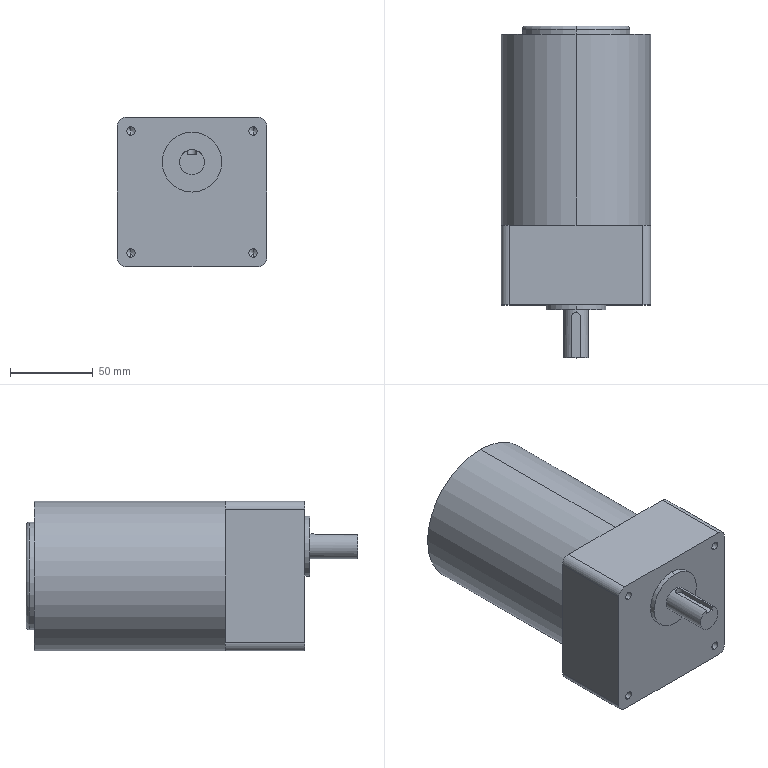Part | SolidWorks | features ICE 6, Fillet 2, CirPattern 1, Extrusion 1, HoleWzd 1, RefAxis 1 | 1 solid | 47 faces | box 90 x 200 x 90 mm | volume 1142205 mm3 | cylinder 21 | plane 16 | cone 8 | torus 2 | commonest cylinder face diameters 5 x9 10 x4 15 x2 36 x2 65 x2 90 x2
STEP:
#1=CARTESIAN_POINT('',(0.,166.,-32.5));
#2=VERTEX_POINT('',#1);
#3=CARTESIAN_POINT('',(0.,166.,32.5));
#4=VERTEX_POINT('',#3);
#5=CARTESIAN_POINT('',(0.,166.,0.));
#6=DIRECTION('',(0.,-1.,0.));
#7=DIRECTION('',(0.,0.,1.));
#8=AXIS2_PLACEMENT_3D('',#5,#6,#7);
#9=CIRCLE('',#8,32.5);
#10=EDGE_CURVE('',#2,#4,#9,.T.);
#11=ORIENTED_EDGE('',*,*,#10,.F.);
#12=CARTESIAN_POINT('',(0.,168.,-30.5));
#13=VERTEX_POINT('',#12);
#14=CARTESIAN_POINT('',(0.,166.,-30.5));
#15=DIRECTION('',(1.,0.,0.));
#16=DIRECTION('',(0.,0.,-1.));
#17=AXIS2_PLACEMENT_3D('',#14,#15,#16);
#18=CIRCLE('',#17,2.);
#19=EDGE_CURVE('',#2,#13,#18,.T.);
#20=ORIENTED_EDGE('',*,*,#19,.T.);
#21=CARTESIAN_POINT('',(0.,168.,30.5));
#22=VERTEX_POINT('',#21);
#23=CARTESIAN_POINT('',(0.,168.,0.));
#24=DIRECTION('',(0.,1.,0.));
#25=DIRECTION('',(0.,0.,1.));
#26=AXIS2_PLACEMENT_3D('',#23,#24,#25);
#27=CIRCLE('',#26,30.5);
#28=EDGE_CURVE('',#22,#13,#27,.T.);
#29=ORIENTED_EDGE('',*,*,#28,.F.);
#30=CARTESIAN_POINT('',(0.,166.,30.5));
#31=DIRECTION('',(-1.,0.,0.));
#32=DIRECTION('',(0.,0.,1.));
#33=AXIS2_PLACEMENT_3D('',#30,#31,#32);
#34=CIRCLE('',#33,2.);
#35=EDGE_CURVE('',#4,#22,#34,.T.);
#36=ORIENTED_EDGE('',*,*,#35,.F.);
#37=EDGE_LOOP('',(#11,#20,#29,#36));
#38=FACE_OUTER_BOUND('',#37,.T.);
#39=CARTESIAN_POINT('',(0.,166.,0.));
#40=DIRECTION('',(0.,1.,0.));
#41=DIRECTION('',(0.,0.,1.));
#42=AXIS2_PLACEMENT_3D('',#39,#40,#41);
#43=TOROIDAL_SURFACE('',#42,30.5,2.);
#44=ADVANCED_FACE('',(#38),#43,.T.);
#45=CARTESIAN_POINT('',(0.,163.,45.));
#46=VERTEX_POINT('',#45);
#47=CARTESIAN_POINT('',(0.,163.,-45.));
#48=VERTEX_POINT('',#47);
#49=CARTESIAN_POINT('',(0.,163.,0.));
#50=DIRECTION('',(0.,1.,0.));
#51=DIRECTION('',(0.,0.,1.));
#52=AXIS2_PLACEMENT_3D('',#49,#50,#51);
#53=CIRCLE('',#52,45.);
#54=EDGE_CURVE('',#46,#48,#53,.T.);
#55=ORIENTED_EDGE('',*,*,#54,.F.);
#56=CARTESIAN_POINT('',(0.,48.,45.));
#57=VERTEX_POINT('',#56);
#58=CARTESIAN_POINT('',(0.,163.,45.));
#59=DIRECTION('',(0.,-1.,0.));
#60=VECTOR('',#59,1000.);
#61=LINE('',#58,#60);
#62=EDGE_CURVE('',#46,#57,#61,.T.);
#63=ORIENTED_EDGE('',*,*,#62,.T.);
#64=CARTESIAN_POINT('',(45.,48.,0.));
#65=VERTEX_POINT('',#64);
#66=CARTESIAN_POINT('',(0.,48.,0.));
#67=DIRECTION('',(0.,1.,0.));
#68=DIRECTION('',(0.,0.,1.));
#69=AXIS2_PLACEMENT_3D('',#66,#67,#68);
#70=CIRCLE('',#69,45.);
#71=EDGE_CURVE('',#57,#65,#70,.T.);
#72=ORIENTED_EDGE('',*,*,#71,.T.);
#73=CARTESIAN_POINT('',(0.,48.,-45.));
#74=VERTEX_POINT('',#73);
#75=CARTESIAN_POINT('',(0.,48.,0.));
#76=DIRECTION('',(0.,1.,0.));
#77=DIRECTION('',(0.,0.,1.));
#78=AXIS2_PLACEMENT_3D('',#75,#76,#77);
#79=CIRCLE('',#78,45.);
#80=EDGE_CURVE('',#65,#74,#79,.T.);
#81=ORIENTED_EDGE('',*,*,#80,.T.);
#82=CARTESIAN_POINT('',(0.,163.,-45.));
#83=DIRECTION('',(0.,-1.,0.));
#84=VECTOR('',#83,1000.);
#85=LINE('',#82,#84);
#86=EDGE_CURVE('',#48,#74,#85,.T.);
#87=ORIENTED_EDGE('',*,*,#86,.F.);
#88=EDGE_LOOP('',(#55,#63,#72,#81,#87));
#89=FACE_OUTER_BOUND('',#88,.T.);
#90=CARTESIAN_POINT('',(0.,163.,0.));
#91=DIRECTION('',(0.,-1.,0.));
#92=DIRECTION('',(0.,0.,-1.));
#93=AXIS2_PLACEMENT_3D('',#90,#91,#92);
#94=CYLINDRICAL_SURFACE('',#93,45.);
#95=ADVANCED_FACE('',(#89),#94,.T.);
#96=ORIENTED_EDGE('',*,*,#10,.T.);
#97=CARTESIAN_POINT('',(0.,163.,32.5));
#98=VERTEX_POINT('',#97);
#99=CARTESIAN_POINT('',(0.,168.,32.5));
#100=DIRECTION('',(0.,-1.,0.));
#101=VECTOR('',#100,1000.);
#102=LINE('',#99,#101);
#103=EDGE_CURVE('',#4,#98,#102,.T.);
#104=ORIENTED_EDGE('',*,*,#103,.T.);
#105=CARTESIAN_POINT('',(0.,163.,-32.5));
#106=VERTEX_POINT('',#105);
#107=CARTESIAN_POINT('',(0.,163.,0.));
#108=DIRECTION('',(0.,1.,0.));
#109=DIRECTION('',(0.,0.,1.));
#110=AXIS2_PLACEMENT_3D('',#107,#108,#109);
#111=CIRCLE('',#110,32.5);
#112=EDGE_CURVE('',#98,#106,#111,.T.);
#113=ORIENTED_EDGE('',*,*,#112,.T.);
#114=CARTESIAN_POINT('',(0.,168.,-32.5));
#115=DIRECTION('',(0.,-1.,0.));
#116=VECTOR('',#115,1000.);
#117=LINE('',#114,#116);
#118=EDGE_CURVE('',#2,#106,#117,.T.);
#119=ORIENTED_EDGE('',*,*,#118,.F.);
#120=EDGE_LOOP('',(#96,#104,#113,#119));
#121=FACE_OUTER_BOUND('',#120,.T.);
#122=CARTESIAN_POINT('',(0.,168.,0.));
#123=DIRECTION('',(0.,-1.,0.));
#124=DIRECTION('',(0.,0.,-1.));
#125=AXIS2_PLACEMENT_3D('',#122,#123,#124);
#126=CYLINDRICAL_SURFACE('',#125,32.5);
#127=ADVANCED_FACE('',(#121),#126,.T.);
#128=CARTESIAN_POINT('',(-36.77,17.,39.27));
#129=VERTEX_POINT('',#128);
#130=CARTESIAN_POINT('',(-36.77,17.,34.27));
#131=VERTEX_POINT('',#130);
#132=CARTESIAN_POINT('',(-36.77,17.,36.77));
#133=DIRECTION('',(0.,-1.,0.));
#134=DIRECTION('',(0.,0.,-1.));
#135=AXIS2_PLACEMENT_3D('',#132,#133,#134);
#136=CIRCLE('',#135,2.5);
#137=EDGE_CURVE('',#129,#131,#136,.T.);
#138=ORIENTED_EDGE('',*,*,#137,.F.);
#139=CARTESIAN_POINT('',(-36.77,0.,39.27));
#140=VERTEX_POINT('',#139);
#141=CARTESIAN_POINT('',(-36.77,0.,39.27));
#142=DIRECTION('',(0.,-1.,0.));
#143=VECTOR('',#142,1000.);
#144=LINE('',#141,#143);
#145=EDGE_CURVE('',#129,#140,#144,.T.);
#146=ORIENTED_EDGE('',*,*,#145,.T.);
#147=CARTESIAN_POINT('',(-36.77,0.,34.27));
#148=VERTEX_POINT('',#147);
#149=CARTESIAN_POINT('',(-36.77,0.,36.77));
#150=DIRECTION('',(0.,-1.,0.));
#151=DIRECTION('',(0.,0.,-1.));
#152=AXIS2_PLACEMENT_3D('',#149,#150,#151);
#153=CIRCLE('',#152,2.5);
#154=EDGE_CURVE('',#140,#148,#153,.T.);
#155=ORIENTED_EDGE('',*,*,#154,.T.);
#156=CARTESIAN_POINT('',(-36.77,0.,34.27));
#157=DIRECTION('',(0.,-1.,0.));
#158=VECTOR('',#157,1000.);
#159=LINE('',#156,#158);
#160=EDGE_CURVE('',#131,#148,#159,.T.);
#161=ORIENTED_EDGE('',*,*,#160,.F.);
#162=EDGE_LOOP('',(#138,#146,#155,#161));
#163=FACE_OUTER_BOUND('',#162,.T.);
#164=CARTESIAN_POINT('',(-36.77,0.,36.77));
#165=DIRECTION('',(0.,-1.,0.));
#166=DIRECTION('',(0.,0.,-1.));
#167=AXIS2_PLACEMENT_3D('',#164,#165,#166);
#168=CYLINDRICAL_SURFACE('',#167,2.5);
#169=ADVANCED_FACE('',(#163),#168,.F.);
#170=CARTESIAN_POINT('',(-36.77,18.502,36.77));
#171=VERTEX_POINT('',#170);
#172=CARTESIAN_POINT('',(-36.77,17.,34.27));
#173=DIRECTION('',(0.,-0.515,-0.8572));
#174=VECTOR('',#173,1000.);
#175=LINE('',#172,#174);
#176=EDGE_CURVE('',#171,#131,#175,.T.);
#177=ORIENTED_EDGE('',*,*,#176,.F.);
#178=CARTESIAN_POINT('',(-36.77,17.,39.27));
#179=DIRECTION('',(0.,-0.515,0.8572));
#180=VECTOR('',#179,1000.);
#181=LINE('',#178,#180);
#182=EDGE_CURVE('',#171,#129,#181,.T.);
#183=ORIENTED_EDGE('',*,*,#182,.T.);
#184=ORIENTED_EDGE('',*,*,#137,.T.);
#185=EDGE_LOOP('',(#177,#183,#184));
#186=FACE_OUTER_BOUND('',#185,.T.);
#187=CARTESIAN_POINT('',(-36.77,17.,36.77));
#188=DIRECTION('',(0.,-1.,0.));
#189=DIRECTION('',(0.,0.,-1.));
#190=AXIS2_PLACEMENT_3D('',#187,#188,#189);
#191=CONICAL_SURFACE('',#190,2.5,1.03);
#192=ADVANCED_FACE('',(#186),#191,.F.);
#193=CARTESIAN_POINT('',(-36.77,17.,-34.27));
#194=VERTEX_POINT('',#193);
#195=CARTESIAN_POINT('',(-36.77,17.,-39.27));
#196=VERTEX_POINT('',#195);
#197=CARTESIAN_POINT('',(-36.77,17.,-36.77));
#198=DIRECTION('',(0.,-1.,0.));
#199=DIRECTION('',(0.,0.,-1.));
#200=AXIS2_PLACEMENT_3D('',#197,#198,#199);
#201=CIRCLE('',#200,2.5);
#202=EDGE_CURVE('',#194,#196,#201,.T.);
#203=ORIENTED_EDGE('',*,*,#202,.F.);
#204=CARTESIAN_POINT('',(-36.77,0.,-34.27));
#205=VERTEX_POINT('',#204);
#206=CARTESIAN_POINT('',(-36.77,0.,-34.27));
#207=DIRECTION('',(0.,-1.,0.));
#208=VECTOR('',#207,1000.);
#209=LINE('',#206,#208);
#210=EDGE_CURVE('',#194,#205,#209,.T.);
#211=ORIENTED_EDGE('',*,*,#210,.T.);
#212=CARTESIAN_POINT('',(-36.77,0.,-39.27));
#213=VERTEX_POINT('',#212);
#214=CARTESIAN_POINT('',(-36.77,0.,-36.77));
#215=DIRECTION('',(0.,-1.,0.));
#216=DIRECTION('',(0.,0.,-1.));
#217=AXIS2_PLACEMENT_3D('',#214,#215,#216);
#218=CIRCLE('',#217,2.5);
#219=EDGE_CURVE('',#205,#213,#218,.T.);
#220=ORIENTED_EDGE('',*,*,#219,.T.);
#221=CARTESIAN_POINT('',(-36.77,0.,-39.27));
#222=DIRECTION('',(0.,-1.,0.));
#223=VECTOR('',#222,1000.);
#224=LINE('',#221,#223);
#225=EDGE_CURVE('',#196,#213,#224,.T.);
#226=ORIENTED_EDGE('',*,*,#225,.F.);
#227=EDGE_LOOP('',(#203,#211,#220,#226));
#228=FACE_OUTER_BOUND('',#227,.T.);
#229=CARTESIAN_POINT('',(-36.77,0.,-36.77));
#230=DIRECTION('',(0.,-1.,0.));
#231=DIRECTION('',(0.,0.,-1.));
#232=AXIS2_PLACEMENT_3D('',#229,#230,#231);
#233=CYLINDRICAL_SURFACE('',#232,2.5);
#234=ADVANCED_FACE('',(#228),#233,.F.);
#235=CARTESIAN_POINT('',(-36.77,18.502,-36.77));
#236=VERTEX_POINT('',#235);
#237=CARTESIAN_POINT('',(-36.77,17.,-39.27));
#238=DIRECTION('',(0.,-0.515,-0.8572));
#239=VECTOR('',#238,1000.);
#240=LINE('',#237,#239);
#241=EDGE_CURVE('',#236,#196,#240,.T.);
#242=ORIENTED_EDGE('',*,*,#241,.F.);
#243=CARTESIAN_POINT('',(-36.77,17.,-34.27));
#244=DIRECTION('',(0.,-0.515,0.8572));
#245=VECTOR('',#244,1000.);
#246=LINE('',#243,#245);
#247=EDGE_CURVE('',#236,#194,#246,.T.);
#248=ORIENTED_EDGE('',*,*,#247,.T.);
#249=ORIENTED_EDGE('',*,*,#202,.T.);
#250=EDGE_LOOP('',(#242,#248,#249));
#251=FACE_OUTER_BOUND('',#250,.T.);
#252=CARTESIAN_POINT('',(-36.77,17.,-36.77));
#253=DIRECTION('',(0.,-1.,0.));
#254=DIRECTION('',(0.,0.,-1.));
#255=AXIS2_PLACEMENT_3D('',#252,#253,#254);
#256=CONICAL_SURFACE('',#255,2.5,1.03);
#257=ADVANCED_FACE('',(#251),#256,.F.);
#258=CARTESIAN_POINT('',(36.77,17.,-34.27));
#259=VERTEX_POINT('',#258);
#260=CARTESIAN_POINT('',(36.77,17.,-39.27));
#261=VERTEX_POINT('',#260);
#262=CARTESIAN_POINT('',(36.77,17.,-36.77));
#263=DIRECTION('',(0.,-1.,0.));
#264=DIRECTION('',(0.,0.,-1.));
#265=AXIS2_PLACEMENT_3D('',#262,#263,#264);
#266=CIRCLE('',#265,2.5);
#267=EDGE_CURVE('',#259,#261,#266,.T.);
#268=ORIENTED_EDGE('',*,*,#267,.F.);
#269=CARTESIAN_POINT('',(36.77,0.,-34.27));
#270=VERTEX_POINT('',#269);
#271=CARTESIAN_POINT('',(36.77,0.,-34.27));
#272=DIRECTION('',(0.,-1.,0.));
#273=VECTOR('',#272,1000.);
#274=LINE('',#271,#273);
#275=EDGE_CURVE('',#259,#270,#274,.T.);
#276=ORIENTED_EDGE('',*,*,#275,.T.);
#277=CARTESIAN_POINT('',(36.77,0.,-39.27));
#278=VERTEX_POINT('',#277);
#279=CARTESIAN_POINT('',(36.77,0.,-36.77));
#280=DIRECTION('',(0.,-1.,0.));
#281=DIRECTION('',(0.,0.,-1.));
#282=AXIS2_PLACEMENT_3D('',#279,#280,#281);
#283=CIRCLE('',#282,2.5);
#284=EDGE_CURVE('',#270,#278,#283,.T.);
#285=ORIENTED_EDGE('',*,*,#284,.T.);
#286=CARTESIAN_POINT('',(36.77,0.,-39.27));
#287=DIRECTION('',(0.,-1.,0.));
#288=VECTOR('',#287,1000.);
#289=LINE('',#286,#288);
#290=EDGE_CURVE('',#261,#278,#289,.T.);
#291=ORIENTED_EDGE('',*,*,#290,.F.);
#292=EDGE_LOOP('',(#268,#276,#285,#291));
#293=FACE_OUTER_BOUND('',#292,.T.);
#294=CARTESIAN_POINT('',(36.77,0.,-36.77));
#295=DIRECTION('',(0.,-1.,0.));
#296=DIRECTION('',(0.,0.,-1.));
#297=AXIS2_PLACEMENT_3D('',#294,#295,#296);
#298=CYLINDRICAL_SURFACE('',#297,2.5);
#299=ADVANCED_FACE('',(#293),#298,.F.);
#300=CARTESIAN_POINT('',(36.77,18.502,-36.77));
#301=VERTEX_POINT('',#300);
#302=CARTESIAN_POINT('',(36.77,17.,-39.27));
#303=DIRECTION('',(0.,-0.515,-0.8572));
#304=VECTOR('',#303,1000.);
#305=LINE('',#302,#304);
#306=EDGE_CURVE('',#301,#261,#305,.T.);
#307=ORIENTED_EDGE('',*,*,#306,.F.);
#308=CARTESIAN_POINT('',(36.77,17.,-34.27));
#309=DIRECTION('',(0.,-0.515,0.8572));
#310=VECTOR('',#309,1000.);
#311=LINE('',#308,#310);
#312=EDGE_CURVE('',#301,#259,#311,.T.);
#313=ORIENTED_EDGE('',*,*,#312,.T.);
#314=ORIENTED_EDGE('',*,*,#267,.T.);
#315=EDGE_LOOP('',(#307,#313,#314));
#316=FACE_OUTER_BOUND('',#315,.T.);
#317=CARTESIAN_POINT('',(36.77,17.,-36.77));
#318=DIRECTION('',(0.,-1.,0.));
#319=DIRECTION('',(0.,0.,-1.));
#320=AXIS2_PLACEMENT_3D('',#317,#318,#319);
#321=CONICAL_SURFACE('',#320,2.5,1.03);
#322=ADVANCED_FACE('',(#316),#321,.F.);
#323=CARTESIAN_POINT('',(36.77,17.,39.27));
#324=VERTEX_POINT('',#323);
#325=CARTESIAN_POINT('',(36.77,17.,34.27));
#326=VERTEX_POINT('',#325);
#327=CARTESIAN_POINT('',(36.77,17.,36.77));
#328=DIRECTION('',(0.,-1.,0.));
#329=DIRECTION('',(0.,0.,-1.));
#330=AXIS2_PLACEMENT_3D('',#327,#328,#329);
#331=CIRCLE('',#330,2.5);
#332=EDGE_CURVE('',#324,#326,#331,.T.);
#333=ORIENTED_EDGE('',*,*,#332,.F.);
#334=CARTESIAN_POINT('',(36.77,0.,39.27));
#335=VERTEX_POINT('',#334);
#336=CARTESIAN_POINT('',(36.77,0.,39.27));
#337=DIRECTION('',(0.,-1.,0.));
#338=VECTOR('',#337,1000.);
#339=LINE('',#336,#338);
#340=EDGE_CURVE('',#324,#335,#339,.T.);
#341=ORIENTED_EDGE('',*,*,#340,.T.);
#342=CARTESIAN_POINT('',(36.77,0.,34.27));
#343=VERTEX_POINT('',#342);
#344=CARTESIAN_POINT('',(36.77,0.,36.77));
#345=DIRECTION('',(0.,-1.,0.));
#346=DIRECTION('',(0.,0.,-1.));
#347=AXIS2_PLACEMENT_3D('',#344,#345,#346);
#348=CIRCLE('',#347,2.5);
#349=EDGE_CURVE('',#335,#343,#348,.T.);
#350=ORIENTED_EDGE('',*,*,#349,.T.);
#351=CARTESIAN_POINT('',(36.77,0.,34.27));
#352=DIRECTION('',(0.,-1.,0.));
#353=VECTOR('',#352,1000.);
#354=LINE('',#351,#353);
#355=EDGE_CURVE('',#326,#343,#354,.T.);
#356=ORIENTED_EDGE('',*,*,#355,.F.);
#357=EDGE_LOOP('',(#333,#341,#350,#356));
#358=FACE_OUTER_BOUND('',#357,.T.);
#359=CARTESIAN_POINT('',(36.77,0.,36.77));
#360=DIRECTION('',(0.,-1.,0.));
#361=DIRECTION('',(0.,0.,-1.));
#362=AXIS2_PLACEMENT_3D('',#359,#360,#361);
#363=CYLINDRICAL_SURFACE('',#362,2.5);
#364=ADVANCED_FACE('',(#358),#363,.F.);
#365=CARTESIAN_POINT('',(36.77,18.502,36.77));
#366=VERTEX_POINT('',#365);
#367=CARTESIAN_POINT('',(36.77,17.,34.27));
#368=DIRECTION('',(0.,-0.515,-0.8572));
#369=VECTOR('',#368,1000.);
#370=LINE('',#367,#369);
#371=EDGE_CURVE('',#366,#326,#370,.T.);
#372=ORIENTED_EDGE('',*,*,#371,.F.);
#373=CARTESIAN_POINT('',(36.77,17.,39.27));
#374=DIRECTION('',(0.,-0.515,0.8572));
#375=VECTOR('',#374,1000.);
#376=LINE('',#373,#375);
#377=EDGE_CURVE('',#366,#324,#376,.T.);
#378=ORIENTED_EDGE('',*,*,#377,.T.);
#379=ORIENTED_EDGE('',*,*,#332,.T.);
#380=EDGE_LOOP('',(#372,#378,#379));
#381=FACE_OUTER_BOUND('',#380,.T.);
#382=CARTESIAN_POINT('',(36.77,17.,36.77));
#383=DIRECTION('',(0.,-1.,0.));
#384=DIRECTION('',(0.,0.,-1.));
#385=AXIS2_PLACEMENT_3D('',#382,#383,#384);
#386=CONICAL_SURFACE('',#385,2.5,1.03);
#387=ADVANCED_FACE('',(#381),#386,.F.);
#388=CARTESIAN_POINT('',(0.,-32.,10.5));
#389=VERTEX_POINT('',#388);
#390=CARTESIAN_POINT('',(2.5,-32.,25.071));
#391=VERTEX_POINT('',#390);
#392=CARTESIAN_POINT('',(0.,-32.,18.));
#393=DIRECTION('',(0.,-1.,0.));
#394=DIRECTION('',(0.,0.,-1.));
#395=AXIS2_PLACEMENT_3D('',#392,#393,#394);
#396=CIRCLE('',#395,7.5);
#397=EDGE_CURVE('',#389,#391,#396,.T.);
#398=ORIENTED_EDGE('',*,*,#397,.F.);
#399=CARTESIAN_POINT('',(0.,-3.,10.5));
#400=VERTEX_POINT('',#399);
#401=CARTESIAN_POINT('',(0.,-32.,10.5));
#402=DIRECTION('',(0.,1.,0.));
#403=VECTOR('',#402,1000.);
#404=LINE('',#401,#403);
#405=EDGE_CURVE('',#389,#400,#404,.T.);
#406=ORIENTED_EDGE('',*,*,#405,.T.);
#407=CARTESIAN_POINT('',(0.,-3.,25.5));
#408=VERTEX_POINT('',#407);
#409=CARTESIAN_POINT('',(0.,-3.,18.));
#410=DIRECTION('',(0.,-1.,0.));
#411=DIRECTION('',(0.,0.,-1.));
#412=AXIS2_PLACEMENT_3D('',#409,#410,#411);
#413=CIRCLE('',#412,7.5);
#414=EDGE_CURVE('',#400,#408,#413,.T.);
#415=ORIENTED_EDGE('',*,*,#414,.T.);
#416=CARTESIAN_POINT('',(0.,-4.5,25.5));
#417=VERTEX_POINT('',#416);
#418=CARTESIAN_POINT('',(0.,-32.,25.5));
#419=DIRECTION('',(0.,1.,0.));
#420=VECTOR('',#419,1000.);
#421=LINE('',#418,#420);
#422=EDGE_CURVE('',#417,#408,#421,.T.);
#423=ORIENTED_EDGE('',*,*,#422,.F.);
#424=CARTESIAN_POINT('',(2.5,-7.,25.071));
#425=VERTEX_POINT('',#424);
#426=CARTESIAN_POINT('',(0.,-4.5,25.5));
#427=CARTESIAN_POINT('',(0.1643,-4.5,25.5));
#428=CARTESIAN_POINT('',(0.3311,-4.517,25.494));
#429=CARTESIAN_POINT('',(0.6524,-4.581,25.473));
#430=CARTESIAN_POINT('',(0.8088,-4.629,25.458));
#431=CARTESIAN_POINT('',(1.113,-4.755,25.419));
#432=CARTESIAN_POINT('',(1.257,-4.833,25.395));
#433=CARTESIAN_POINT('',(1.526,-5.013,25.344));
#434=CARTESIAN_POINT('',(1.653,-5.118,25.316));
#435=CARTESIAN_POINT('',(1.883,-5.348,25.261));
#436=CARTESIAN_POINT('',(1.986,-5.473,25.233));
#437=CARTESIAN_POINT('',(2.167,-5.742,25.181));
#438=CARTESIAN_POINT('',(2.245,-5.888,25.156));
#439=CARTESIAN_POINT('',(2.37,-6.189,25.116));
#440=CARTESIAN_POINT('',(2.418,-6.344,25.1));
#441=CARTESIAN_POINT('',(2.483,-6.668,25.077));
#442=CARTESIAN_POINT('',(2.5,-6.834,25.071));
#443=CARTESIAN_POINT('',(2.5,-7.,25.071));
#444=B_SPLINE_CURVE_WITH_KNOTS('',3,(#426,#427,#428,#429,#430,#431,#432,#433,#434,#435,#436,#437,#438,#439,#440,#441,#442,#443),.UNSPECIFIED.,.F.,.F.,(4,2,2,2,2,2,2,2,4),(0.003937,0.004429,0.004921,0.005412,0.005904,0.006395,0.006887,0.007378,0.00787),.UNSPECIFIED.);
#445=EDGE_CURVE('',#417,#425,#444,.T.);
#446=ORIENTED_EDGE('',*,*,#445,.T.);
#447=CARTESIAN_POINT('',(2.5,-32.,25.071));
#448=DIRECTION('',(0.,-1.,0.));
#449=VECTOR('',#448,1000.);
#450=LINE('',#447,#449);
#451=EDGE_CURVE('',#425,#391,#450,.T.);
#452=ORIENTED_EDGE('',*,*,#451,.T.);
#453=EDGE_LOOP('',(#398,#406,#415,#423,#446,#452));
#454=FACE_OUTER_BOUND('',#453,.T.);
#455=CARTESIAN_POINT('',(0.,-32.,18.));
#456=DIRECTION('',(0.,1.,0.));
#457=DIRECTION('',(0.,0.,1.));
#458=AXIS2_PLACEMENT_3D('',#455,#456,#457);
#459=CYLINDRICAL_SURFACE('',#458,7.5);
#460=ADVANCED_FACE('',(#454),#459,.T.);
#461=CARTESIAN_POINT('',(0.,-3.,0.));
#462=VERTEX_POINT('',#461);
#463=CARTESIAN_POINT('',(0.,-3.,36.));
#464=VERTEX_POINT('',#463);
#465=CARTESIAN_POINT('',(0.,-3.,18.));
#466=DIRECTION('',(0.,-1.,0.));
#467=DIRECTION('',(0.,0.,-1.));
#468=AXIS2_PLACEMENT_3D('',#465,#466,#467);
#469=CIRCLE('',#468,18.);
#470=EDGE_CURVE('',#462,#464,#469,.T.);
#471=ORIENTED_EDGE('',*,*,#470,.F.);
#472=CARTESIAN_POINT('',(0.,0.,0.));
#473=VERTEX_POINT('',#472);
#474=CARTESIAN_POINT('',(0.,-3.,0.));
#475=DIRECTION('',(0.,1.,0.));
#476=VECTOR('',#475,1000.);
#477=LINE('',#474,#476);
#478=EDGE_CURVE('',#462,#473,#477,.T.);
#479=ORIENTED_EDGE('',*,*,#478,.T.);
#480=CARTESIAN_POINT('',(0.,0.,36.));
#481=VERTEX_POINT('',#480);
#482=CARTESIAN_POINT('',(0.,0.,18.));
#483=DIRECTION('',(0.,-1.,0.));
#484=DIRECTION('',(0.,0.,1.));
#485=AXIS2_PLACEMENT_3D('',#482,#483,#484);
#486=CIRCLE('',#485,18.);
#487=EDGE_CURVE('',#473,#481,#486,.T.);
#488=ORIENTED_EDGE('',*,*,#487,.T.);
#489=CARTESIAN_POINT('',(0.,-3.,36.));
#490=DIRECTION('',(0.,1.,0.));
#491=VECTOR('',#490,1000.);
#492=LINE('',#489,#491);
#493=EDGE_CURVE('',#464,#481,#492,.T.);
#494=ORIENTED_EDGE('',*,*,#493,.F.);
#495=EDGE_LOOP('',(#471,#479,#488,#494));
#496=FACE_OUTER_BOUND('',#495,.T.);
#497=CARTESIAN_POINT('',(0.,-3.,18.));
#498=DIRECTION('',(0.,1.,0.));
#499=DIRECTION('',(0.,0.,1.));
#500=AXIS2_PLACEMENT_3D('',#497,#498,#499);
#501=CYLINDRICAL_SURFACE('',#500,18.);
#502=ADVANCED_FACE('',(#496),#501,.T.);
#503=CARTESIAN_POINT('',(0.,-3.,18.));
#504=DIRECTION('',(0.,-1.,0.));
#505=DIRECTION('',(0.,0.,-1.));
#506=AXIS2_PLACEMENT_3D('',#503,#504,#505);
#507=CIRCLE('',#506,18.);
#508=EDGE_CURVE('',#464,#462,#507,.T.);
#509=ORIENTED_EDGE('',*,*,#508,.T.);
#510=ORIENTED_EDGE('',*,*,#470,.T.);
#511=EDGE_LOOP('',(#509,#510));
#512=FACE_OUTER_BOUND('',#511,.T.);
#513=CARTESIAN_POINT('',(0.,-3.,18.));
#514=DIRECTION('',(0.,-1.,0.));
#515=DIRECTION('',(0.,0.,-1.));
#516=AXIS2_PLACEMENT_3D('',#513,#514,#515);
#517=CIRCLE('',#516,7.5);
#518=EDGE_CURVE('',#408,#400,#517,.T.);
#519=ORIENTED_EDGE('',*,*,#518,.F.);
#520=ORIENTED_EDGE('',*,*,#414,.F.);
#521=EDGE_LOOP('',(#519,#520));
#522=FACE_BOUND('',#521,.T.);
#523=CARTESIAN_POINT('',(0.,-3.,18.));
#524=DIRECTION('',(0.,-1.,0.));
#525=DIRECTION('',(0.,0.,-1.));
#526=AXIS2_PLACEMENT_3D('',#523,#524,#525);
#527=PLANE('',#526);
#528=ADVANCED_FACE('',(#512,#522),#527,.T.);
#529=CARTESIAN_POINT('',(-36.77,0.,36.77));
#530=DIRECTION('',(0.,-1.,0.));
#531=DIRECTION('',(0.,0.,-1.));
#532=AXIS2_PLACEMENT_3D('',#529,#530,#531);
#533=CIRCLE('',#532,2.5);
#534=EDGE_CURVE('',#148,#140,#533,.T.);
#535=ORIENTED_EDGE('',*,*,#534,.F.);
#536=ORIENTED_EDGE('',*,*,#154,.F.);
#537=EDGE_LOOP('',(#535,#536));
#538=FACE_BOUND('',#537,.T.);
#539=CARTESIAN_POINT('',(-36.77,0.,-36.77));
#540=DIRECTION('',(0.,-1.,0.));
#541=DIRECTION('',(0.,0.,-1.));
#542=AXIS2_PLACEMENT_3D('',#539,#540,#541);
#543=CIRCLE('',#542,2.5);
#544=EDGE_CURVE('',#213,#205,#543,.T.);
#545=ORIENTED_EDGE('',*,*,#544,.F.);
#546=ORIENTED_EDGE('',*,*,#219,.F.);
#547=EDGE_LOOP('',(#545,#546));
#548=FACE_BOUND('',#547,.T.);
#549=CARTESIAN_POINT('',(36.77,0.,-36.77));
#550=DIRECTION('',(0.,-1.,0.));
#551=DIRECTION('',(0.,0.,-1.));
#552=AXIS2_PLACEMENT_3D('',#549,#550,#551);
#553=CIRCLE('',#552,2.5);
#554=EDGE_CURVE('',#278,#270,#553,.T.);
#555=ORIENTED_EDGE('',*,*,#554,.F.);
#556=ORIENTED_EDGE('',*,*,#284,.F.);
#557=EDGE_LOOP('',(#555,#556));
#558=FACE_BOUND('',#557,.T.);
#559=CARTESIAN_POINT('',(36.77,0.,36.77));
#560=DIRECTION('',(0.,-1.,0.));
#561=DIRECTION('',(0.,0.,-1.));
#562=AXIS2_PLACEMENT_3D('',#559,#560,#561);
#563=CIRCLE('',#562,2.5);
#564=EDGE_CURVE('',#343,#335,#563,.T.);
#565=ORIENTED_EDGE('',*,*,#564,.F.);
#566=ORIENTED_EDGE('',*,*,#349,.F.);
#567=EDGE_LOOP('',(#565,#566));
#568=FACE_BOUND('',#567,.T.);
#569=CARTESIAN_POINT('',(-40.,0.,45.));
#570=VERTEX_POINT('',#569);
#571=CARTESIAN_POINT('',(40.,0.,45.));
#572=VERTEX_POINT('',#571);
#573=CARTESIAN_POINT('',(-45.,0.,45.));
#574=DIRECTION('',(1.,0.,0.));
#575=VECTOR('',#574,1000.);
#576=LINE('',#573,#575);
#577=EDGE_CURVE('',#570,#572,#576,.T.);
#578=ORIENTED_EDGE('',*,*,#577,.F.);
#579=CARTESIAN_POINT('',(-45.,0.,40.));
#580=VERTEX_POINT('',#579);
#581=CARTESIAN_POINT('',(-40.,0.,40.));
#582=DIRECTION('',(0.,-1.,0.));
#583=DIRECTION('',(0.,0.,1.));
#584=AXIS2_PLACEMENT_3D('',#581,#582,#583);
#585=CIRCLE('',#584,5.);
#586=EDGE_CURVE('',#570,#580,#585,.T.);
#587=ORIENTED_EDGE('',*,*,#586,.T.);
#588=CARTESIAN_POINT('',(-45.,0.,-40.));
#589=VERTEX_POINT('',#588);
#590=CARTESIAN_POINT('',(-45.,0.,-45.));
#591=DIRECTION('',(0.,0.,1.));
#592=VECTOR('',#591,1000.);
#593=LINE('',#590,#592);
#594=EDGE_CURVE('',#589,#580,#593,.T.);
#595=ORIENTED_EDGE('',*,*,#594,.F.);
#596=CARTESIAN_POINT('',(-40.,0.,-45.));
#597=VERTEX_POINT('',#596);
#598=CARTESIAN_POINT('',(-40.,0.,-40.));
#599=DIRECTION('',(0.,-1.,0.));
#600=DIRECTION('',(0.,0.,1.));
#601=AXIS2_PLACEMENT_3D('',#598,#599,#600);
#602=CIRCLE('',#601,5.);
#603=EDGE_CURVE('',#589,#597,#602,.T.);
#604=ORIENTED_EDGE('',*,*,#603,.T.);
#605=CARTESIAN_POINT('',(40.,0.,-45.));
#606=VERTEX_POINT('',#605);
#607=CARTESIAN_POINT('',(-45.,0.,-45.));
#608=DIRECTION('',(-1.,0.,0.));
#609=VECTOR('',#608,1000.);
#610=LINE('',#607,#609);
#611=EDGE_CURVE('',#606,#597,#610,.T.);
#612=ORIENTED_EDGE('',*,*,#611,.F.);
#613=CARTESIAN_POINT('',(45.,0.,-40.));
#614=VERTEX_POINT('',#613);
#615=CARTESIAN_POINT('',(40.,0.,-40.));
#616=DIRECTION('',(0.,-1.,0.));
#617=DIRECTION('',(0.,0.,1.));
#618=AXIS2_PLACEMENT_3D('',#615,#616,#617);
#619=CIRCLE('',#618,5.);
#620=EDGE_CURVE('',#606,#614,#619,.T.);
#621=ORIENTED_EDGE('',*,*,#620,.T.);
#622=CARTESIAN_POINT('',(45.,0.,40.));
#623=VERTEX_POINT('',#622);
#624=CARTESIAN_POINT('',(45.,0.,-45.));
#625=DIRECTION('',(0.,0.,-1.));
#626=VECTOR('',#625,1000.);
#627=LINE('',#624,#626);
#628=EDGE_CURVE('',#623,#614,#627,.T.);
#629=ORIENTED_EDGE('',*,*,#628,.F.);
#630=CARTESIAN_POINT('',(40.,0.,40.));
#631=DIRECTION('',(0.,-1.,0.));
#632=DIRECTION('',(0.,0.,1.));
#633=AXIS2_PLACEMENT_3D('',#630,#631,#632);
#634=CIRCLE('',#633,5.);
#635=EDGE_CURVE('',#623,#572,#634,.T.);
#636=ORIENTED_EDGE('',*,*,#635,.T.);
#637=EDGE_LOOP('',(#578,#587,#595,#604,#612,#621,#629,#636));
#638=FACE_OUTER_BOUND('',#637,.T.);
#639=CARTESIAN_POINT('',(0.,0.,18.));
#640=DIRECTION('',(0.,-1.,0.));
#641=DIRECTION('',(0.,0.,1.));
#642=AXIS2_PLACEMENT_3D('',#639,#640,#641);
#643=CIRCLE('',#642,18.);
#644=EDGE_CURVE('',#481,#473,#643,.T.);
#645=ORIENTED_EDGE('',*,*,#644,.F.);
#646=ORIENTED_EDGE('',*,*,#487,.F.);
#647=EDGE_LOOP('',(#645,#646));
#648=FACE_BOUND('',#647,.T.);
#649=CARTESIAN_POINT('',(-45.,0.,45.));
#650=DIRECTION('',(0.,1.,0.));
#651=DIRECTION('',(0.,0.,1.));
#652=AXIS2_PLACEMENT_3D('',#649,#650,#651);
#653=PLANE('',#652);
#654=ADVANCED_FACE('',(#538,#548,#558,#568,#638,#648),#653,.F.);
#655=ORIENTED_EDGE('',*,*,#594,.T.);
#656=CARTESIAN_POINT('',(-45.,48.,40.));
#657=VERTEX_POINT('',#656);
#658=CARTESIAN_POINT('',(-45.,43.,40.));
#659=DIRECTION('',(0.,1.,0.));
#660=VECTOR('',#659,1000.);
#661=LINE('',#658,#660);
#662=EDGE_CURVE('',#580,#657,#661,.T.);
#663=ORIENTED_EDGE('',*,*,#662,.T.);
#664=CARTESIAN_POINT('',(-45.,48.,0.));
#665=VERTEX_POINT('',#664);
#666=CARTESIAN_POINT('',(-45.,48.,-45.));
#667=DIRECTION('',(0.,0.,1.));
#668=VECTOR('',#667,1000.);
#669=LINE('',#666,#668);
#670=EDGE_CURVE('',#665,#657,#669,.T.);
#671=ORIENTED_EDGE('',*,*,#670,.F.);
#672=CARTESIAN_POINT('',(-45.,48.,-40.));
#673=VERTEX_POINT('',#672);
#674=CARTESIAN_POINT('',(-45.,48.,-45.));
#675=DIRECTION('',(0.,0.,1.));
#676=VECTOR('',#675,1000.);
#677=LINE('',#674,#676);
#678=EDGE_CURVE('',#673,#665,#677,.T.);
#679=ORIENTED_EDGE('',*,*,#678,.F.);
#680=CARTESIAN_POINT('',(-45.,43.,-40.));
#681=DIRECTION('',(0.,-1.,0.));
#682=VECTOR('',#681,1000.);
#683=LINE('',#680,#682);
#684=EDGE_CURVE('',#673,#589,#683,.T.);
#685=ORIENTED_EDGE('',*,*,#684,.T.);
#686=EDGE_LOOP('',(#655,#663,#671,#679,#685));
#687=FACE_OUTER_BOUND('',#686,.T.);
#688=CARTESIAN_POINT('',(-45.,43.,-45.));
#689=DIRECTION('',(1.,0.,0.));
#690=DIRECTION('',(0.,0.,-1.));
#691=AXIS2_PLACEMENT_3D('',#688,#689,#690);
#692=PLANE('',#691);
#693=ADVANCED_FACE('',(#687),#692,.F.);
#694=CARTESIAN_POINT('',(-40.,48.,45.));
#695=VERTEX_POINT('',#694);
#696=CARTESIAN_POINT('',(-45.,48.,45.));
#697=DIRECTION('',(1.,0.,0.));
#698=VECTOR('',#697,1000.);
#699=LINE('',#696,#698);
#700=EDGE_CURVE('',#695,#57,#699,.T.);
#701=ORIENTED_EDGE('',*,*,#700,.F.);
#702=CARTESIAN_POINT('',(-40.,43.,45.));
#703=DIRECTION('',(0.,-1.,0.));
#704=VECTOR('',#703,1000.);
#705=LINE('',#702,#704);
#706=EDGE_CURVE('',#695,#570,#705,.T.);
#707=ORIENTED_EDGE('',*,*,#706,.T.);
#708=ORIENTED_EDGE('',*,*,#577,.T.);
#709=CARTESIAN_POINT('',(40.,48.,45.));
#710=VERTEX_POINT('',#709);
#711=CARTESIAN_POINT('',(40.,43.,45.));
#712=DIRECTION('',(0.,1.,0.));
#713=VECTOR('',#712,1000.);
#714=LINE('',#711,#713);
#715=EDGE_CURVE('',#572,#710,#714,.T.);
#716=ORIENTED_EDGE('',*,*,#715,.T.);
#717=CARTESIAN_POINT('',(-45.,48.,45.));
#718=DIRECTION('',(1.,0.,0.));
#719=VECTOR('',#718,1000.);
#720=LINE('',#717,#719);
#721=EDGE_CURVE('',#57,#710,#720,.T.);
#722=ORIENTED_EDGE('',*,*,#721,.F.);
#723=EDGE_LOOP('',(#701,#707,#708,#716,#722));
#724=FACE_OUTER_BOUND('',#723,.T.);
#725=CARTESIAN_POINT('',(-45.,43.,45.));
#726=DIRECTION('',(0.,0.,-1.));
#727=DIRECTION('',(-1.,0.,0.));
#728=AXIS2_PLACEMENT_3D('',#725,#726,#727);
#729=PLANE('',#728);
#730=ADVANCED_FACE('',(#724),#729,.F.);
#731=CARTESIAN_POINT('',(45.,48.,40.));
#732=VERTEX_POINT('',#731);
#733=CARTESIAN_POINT('',(45.,48.,-45.));
#734=DIRECTION('',(0.,0.,-1.));
#735=VECTOR('',#734,1000.);
#736=LINE('',#733,#735);
#737=EDGE_CURVE('',#732,#65,#736,.T.);
#738=ORIENTED_EDGE('',*,*,#737,.F.);
#739=CARTESIAN_POINT('',(45.,43.,40.));
#740=DIRECTION('',(0.,-1.,0.));
#741=VECTOR('',#740,1000.);
#742=LINE('',#739,#741);
#743=EDGE_CURVE('',#732,#623,#742,.T.);
#744=ORIENTED_EDGE('',*,*,#743,.T.);
#745=ORIENTED_EDGE('',*,*,#628,.T.);
#746=CARTESIAN_POINT('',(45.,48.,-40.));
#747=VERTEX_POINT('',#746);
#748=CARTESIAN_POINT('',(45.,43.,-40.));
#749=DIRECTION('',(0.,1.,0.));
#750=VECTOR('',#749,1000.);
#751=LINE('',#748,#750);
#752=EDGE_CURVE('',#614,#747,#751,.T.);
#753=ORIENTED_EDGE('',*,*,#752,.T.);
#754=CARTESIAN_POINT('',(45.,48.,-45.));
#755=DIRECTION('',(0.,0.,-1.));
#756=VECTOR('',#755,1000.);
#757=LINE('',#754,#756);
#758=EDGE_CURVE('',#65,#747,#757,.T.);
#759=ORIENTED_EDGE('',*,*,#758,.F.);
#760=EDGE_LOOP('',(#738,#744,#745,#753,#759));
#761=FACE_OUTER_BOUND('',#760,.T.);
#762=CARTESIAN_POINT('',(45.,43.,-45.));
#763=DIRECTION('',(-1.,0.,0.));
#764=DIRECTION('',(0.,0.,1.));
#765=AXIS2_PLACEMENT_3D('',#762,#763,#764);
#766=PLANE('',#765);
#767=ADVANCED_FACE('',(#761),#766,.F.);
#768=ORIENTED_EDGE('',*,*,#611,.T.);
#769=CARTESIAN_POINT('',(-40.,48.,-45.));
#770=VERTEX_POINT('',#769);
#771=CARTESIAN_POINT('',(-40.,43.,-45.));
#772=DIRECTION('',(0.,1.,0.));
#773=VECTOR('',#772,1000.);
#774=LINE('',#771,#773);
#775=EDGE_CURVE('',#597,#770,#774,.T.);
#776=ORIENTED_EDGE('',*,*,#775,.T.);
#777=CARTESIAN_POINT('',(-45.,48.,-45.));
#778=DIRECTION('',(-1.,0.,0.));
#779=VECTOR('',#778,1000.);
#780=LINE('',#777,#779);
#781=EDGE_CURVE('',#74,#770,#780,.T.);
#782=ORIENTED_EDGE('',*,*,#781,.F.);
#783=CARTESIAN_POINT('',(40.,48.,-45.));
#784=VERTEX_POINT('',#783);
#785=CARTESIAN_POINT('',(-45.,48.,-45.));
#786=DIRECTION('',(-1.,0.,0.));
#787=VECTOR('',#786,1000.);
#788=LINE('',#785,#787);
#789=EDGE_CURVE('',#784,#74,#788,.T.);
#790=ORIENTED_EDGE('',*,*,#789,.F.);
#791=CARTESIAN_POINT('',(40.,43.,-45.));
#792=DIRECTION('',(0.,-1.,0.));
#793=VECTOR('',#792,1000.);
#794=LINE('',#791,#793);
#795=EDGE_CURVE('',#784,#606,#794,.T.);
#796=ORIENTED_EDGE('',*,*,#795,.T.);
#797=EDGE_LOOP('',(#768,#776,#782,#790,#796));
#798=FACE_OUTER_BOUND('',#797,.T.);
#799=CARTESIAN_POINT('',(-45.,43.,-45.));
#800=DIRECTION('',(0.,0.,1.));
#801=DIRECTION('',(1.,0.,0.));
#802=AXIS2_PLACEMENT_3D('',#799,#800,#801);
#803=PLANE('',#802);
#804=ADVANCED_FACE('',(#798),#803,.F.);
#805=ORIENTED_EDGE('',*,*,#478,.F.);
#806=ORIENTED_EDGE('',*,*,#508,.F.);
#807=ORIENTED_EDGE('',*,*,#493,.T.);
#808=ORIENTED_EDGE('',*,*,#644,.T.);
#809=EDGE_LOOP('',(#805,#806,#807,#808));
#810=FACE_OUTER_BOUND('',#809,.T.);
#811=CARTESIAN_POINT('',(0.,-3.,18.));
#812=DIRECTION('',(0.,1.,0.));
#813=DIRECTION('',(0.,0.,1.));
#814=AXIS2_PLACEMENT_3D('',#811,#812,#813);
#815=CYLINDRICAL_SURFACE('',#814,18.);
#816=ADVANCED_FACE('',(#810),#815,.T.);
#817=ORIENTED_EDGE('',*,*,#405,.F.);
#818=CARTESIAN_POINT('',(-2.5,-32.,25.071));
#819=VERTEX_POINT('',#818);
#820=CARTESIAN_POINT('',(0.,-32.,18.));
#821=DIRECTION('',(0.,-1.,0.));
#822=DIRECTION('',(0.,0.,-1.));
#823=AXIS2_PLACEMENT_3D('',#820,#821,#822);
#824=CIRCLE('',#823,7.5);
#825=EDGE_CURVE('',#819,#389,#824,.T.);
#826=ORIENTED_EDGE('',*,*,#825,.F.);
#827=CARTESIAN_POINT('',(-2.5,-7.,25.071));
#828=VERTEX_POINT('',#827);
#829=CARTESIAN_POINT('',(-2.5,-32.,25.071));
#830=DIRECTION('',(0.,1.,0.));
#831=VECTOR('',#830,1000.);
#832=LINE('',#829,#831);
#833=EDGE_CURVE('',#819,#828,#832,.T.);
#834=ORIENTED_EDGE('',*,*,#833,.T.);
#835=CARTESIAN_POINT('',(-2.5,-7.,25.071));
#836=CARTESIAN_POINT('',(-2.5,-6.833,25.071));
#837=CARTESIAN_POINT('',(-2.484,-6.67,25.077));
#838=CARTESIAN_POINT('',(-2.419,-6.349,25.099));
#839=CARTESIAN_POINT('',(-2.371,-6.189,25.116));
#840=CARTESIAN_POINT('',(-2.245,-5.887,25.157));
#841=CARTESIAN_POINT('',(-2.168,-5.744,25.181));
#842=CARTESIAN_POINT('',(-1.986,-5.473,25.233));
#843=CARTESIAN_POINT('',(-1.882,-5.346,25.261));
#844=CARTESIAN_POINT('',(-1.538,-5.003,25.344));
#845=CARTESIAN_POINT('',(-1.261,-4.817,25.399));
#846=CARTESIAN_POINT('',(-0.81,-4.629,25.458));
#847=CARTESIAN_POINT('',(-0.6511,-4.581,25.473));
#848=CARTESIAN_POINT('',(-0.3276,-4.516,25.495));
#849=CARTESIAN_POINT('',(-0.1645,-4.5,25.5));
#850=CARTESIAN_POINT('',(0.,-4.5,25.5));
#851=B_SPLINE_CURVE_WITH_KNOTS('',3,(#835,#836,#837,#838,#839,#840,#841,#842,#843,#844,#845,#846,#847,#848,#849,#850),.UNSPECIFIED.,.F.,.F.,(4,2,2,2,2,2,2,4),(0.,0.0004922,0.0009844,0.001477,0.001969,0.002953,0.003445,0.003937),.UNSPECIFIED.);
#852=EDGE_CURVE('',#828,#417,#851,.T.);
#853=ORIENTED_EDGE('',*,*,#852,.T.);
#854=ORIENTED_EDGE('',*,*,#422,.T.);
#855=ORIENTED_EDGE('',*,*,#518,.T.);
#856=EDGE_LOOP('',(#817,#826,#834,#853,#854,#855));
#857=FACE_OUTER_BOUND('',#856,.T.);
#858=CARTESIAN_POINT('',(0.,-32.,18.));
#859=DIRECTION('',(0.,1.,0.));
#860=DIRECTION('',(0.,0.,1.));
#861=AXIS2_PLACEMENT_3D('',#858,#859,#860);
#862=CYLINDRICAL_SURFACE('',#861,7.5);
#863=ADVANCED_FACE('',(#857),#862,.T.);
#864=CARTESIAN_POINT('',(2.5,-32.,22.5));
#865=VERTEX_POINT('',#864);
#866=CARTESIAN_POINT('',(2.5,-32.,22.5));
#867=DIRECTION('',(0.,0.,1.));
#868=VECTOR('',#867,1000.);
#869=LINE('',#866,#868);
#870=EDGE_CURVE('',#865,#391,#869,.T.);
#871=ORIENTED_EDGE('',*,*,#870,.F.);
#872=CARTESIAN_POINT('',(-2.5,-32.,22.5));
#873=VERTEX_POINT('',#872);
#874=CARTESIAN_POINT('',(-2.5,-32.,22.5));
#875=DIRECTION('',(1.,0.,0.));
#876=VECTOR('',#875,1000.);
#877=LINE('',#874,#876);
#878=EDGE_CURVE('',#873,#865,#877,.T.);
#879=ORIENTED_EDGE('',*,*,#878,.F.);
#880=CARTESIAN_POINT('',(-2.5,-32.,22.5));
#881=DIRECTION('',(0.,0.,1.));
#882=VECTOR('',#881,1000.);
#883=LINE('',#880,#882);
#884=EDGE_CURVE('',#873,#819,#883,.T.);
#885=ORIENTED_EDGE('',*,*,#884,.T.);
#886=ORIENTED_EDGE('',*,*,#825,.T.);
#887=ORIENTED_EDGE('',*,*,#397,.T.);
#888=EDGE_LOOP('',(#871,#879,#885,#886,#887));
#889=FACE_OUTER_BOUND('',#888,.T.);
#890=CARTESIAN_POINT('',(0.,-32.,18.));
#891=DIRECTION('',(0.,-1.,0.));
#892=DIRECTION('',(0.,0.,-1.));
#893=AXIS2_PLACEMENT_3D('',#890,#891,#892);
#894=PLANE('',#893);
#895=ADVANCED_FACE('',(#889),#894,.T.);
#896=CARTESIAN_POINT('',(-2.5,-7.,22.5));
#897=VERTEX_POINT('',#896);
#898=CARTESIAN_POINT('',(-2.5,-7.,22.5));
#899=DIRECTION('',(0.,0.,1.));
#900=VECTOR('',#899,1000.);
#901=LINE('',#898,#900);
#902=EDGE_CURVE('',#897,#828,#901,.T.);
#903=ORIENTED_EDGE('',*,*,#902,.F.);
#904=CARTESIAN_POINT('',(2.5,-7.,22.5));
#905=VERTEX_POINT('',#904);
#906=CARTESIAN_POINT('',(0.,-7.,22.5));
#907=DIRECTION('',(0.,0.,1.));
#908=DIRECTION('',(1.,0.,0.));
#909=AXIS2_PLACEMENT_3D('',#906,#907,#908);
#910=CIRCLE('',#909,2.5);
#911=EDGE_CURVE('',#905,#897,#910,.T.);
#912=ORIENTED_EDGE('',*,*,#911,.F.);
#913=CARTESIAN_POINT('',(2.5,-7.,22.5));
#914=DIRECTION('',(0.,0.,1.));
#915=VECTOR('',#914,1000.);
#916=LINE('',#913,#915);
#917=EDGE_CURVE('',#905,#425,#916,.T.);
#918=ORIENTED_EDGE('',*,*,#917,.T.);
#919=ORIENTED_EDGE('',*,*,#445,.F.);
#920=ORIENTED_EDGE('',*,*,#852,.F.);
#921=EDGE_LOOP('',(#903,#912,#918,#919,#920));
#922=FACE_OUTER_BOUND('',#921,.T.);
#923=CARTESIAN_POINT('',(0.,-7.,22.5));
#924=DIRECTION('',(0.,0.,1.));
#925=DIRECTION('',(1.,0.,0.));
#926=AXIS2_PLACEMENT_3D('',#923,#924,#925);
#927=CYLINDRICAL_SURFACE('',#926,2.5);
#928=ADVANCED_FACE('',(#922),#927,.F.);
#929=ORIENTED_EDGE('',*,*,#917,.F.);
#930=CARTESIAN_POINT('',(2.5,-7.,22.5));
#931=DIRECTION('',(0.,1.,0.));
#932=VECTOR('',#931,1000.);
#933=LINE('',#930,#932);
#934=EDGE_CURVE('',#865,#905,#933,.T.);
#935=ORIENTED_EDGE('',*,*,#934,.F.);
#936=ORIENTED_EDGE('',*,*,#870,.T.);
#937=ORIENTED_EDGE('',*,*,#451,.F.);
#938=EDGE_LOOP('',(#929,#935,#936,#937));
#939=FACE_OUTER_BOUND('',#938,.T.);
#940=CARTESIAN_POINT('',(2.5,-7.,22.5));
#941=DIRECTION('',(1.,0.,0.));
#942=DIRECTION('',(0.,1.,0.));
#943=AXIS2_PLACEMENT_3D('',#940,#941,#942);
#944=PLANE('',#943);
#945=ADVANCED_FACE('',(#939),#944,.F.);
#946=ORIENTED_EDGE('',*,*,#884,.F.);
#947=CARTESIAN_POINT('',(-2.5,-7.,22.5));
#948=DIRECTION('',(0.,-1.,0.));
#949=VECTOR('',#948,1000.);
#950=LINE('',#947,#949);
#951=EDGE_CURVE('',#897,#873,#950,.T.);
#952=ORIENTED_EDGE('',*,*,#951,.F.);
#953=ORIENTED_EDGE('',*,*,#902,.T.);
#954=ORIENTED_EDGE('',*,*,#833,.F.);
#955=EDGE_LOOP('',(#946,#952,#953,#954));
#956=FACE_OUTER_BOUND('',#955,.T.);
#957=CARTESIAN_POINT('',(-2.5,-7.,22.5));
#958=DIRECTION('',(-1.,0.,0.));
#959=DIRECTION('',(0.,-1.,0.));
#960=AXIS2_PLACEMENT_3D('',#957,#958,#959);
#961=PLANE('',#960);
#962=ADVANCED_FACE('',(#956),#961,.F.);
#963=ORIENTED_EDGE('',*,*,#911,.T.);
#964=ORIENTED_EDGE('',*,*,#951,.T.);
#965=ORIENTED_EDGE('',*,*,#878,.T.);
#966=ORIENTED_EDGE('',*,*,#934,.T.);
#967=EDGE_LOOP('',(#963,#964,#965,#966));
#968=FACE_OUTER_BOUND('',#967,.T.);
#969=CARTESIAN_POINT('',(0.,-7.,22.5));
#970=DIRECTION('',(0.,0.,1.));
#971=DIRECTION('',(1.,0.,0.));
#972=AXIS2_PLACEMENT_3D('',#969,#970,#971);
#973=PLANE('',#972);
#974=ADVANCED_FACE('',(#968),#973,.T.);
#975=ORIENTED_EDGE('',*,*,#377,.F.);
#976=ORIENTED_EDGE('',*,*,#371,.T.);
#977=CARTESIAN_POINT('',(36.77,17.,36.77));
#978=DIRECTION('',(0.,-1.,0.));
#979=DIRECTION('',(0.,0.,-1.));
#980=AXIS2_PLACEMENT_3D('',#977,#978,#979);
#981=CIRCLE('',#980,2.5);
#982=EDGE_CURVE('',#326,#324,#981,.T.);
#983=ORIENTED_EDGE('',*,*,#982,.T.);
#984=EDGE_LOOP('',(#975,#976,#983));
#985=FACE_OUTER_BOUND('',#984,.T.);
#986=CARTESIAN_POINT('',(36.77,17.,36.77));
#987=DIRECTION('',(0.,-1.,0.));
#988=DIRECTION('',(0.,0.,-1.));
#989=AXIS2_PLACEMENT_3D('',#986,#987,#988);
#990=CONICAL_SURFACE('',#989,2.5,1.03);
#991=ADVANCED_FACE('',(#985),#990,.F.);
#992=ORIENTED_EDGE('',*,*,#340,.F.);
#993=ORIENTED_EDGE('',*,*,#982,.F.);
#994=ORIENTED_EDGE('',*,*,#355,.T.);
#995=ORIENTED_EDGE('',*,*,#564,.T.);
#996=EDGE_LOOP('',(#992,#993,#994,#995));
#997=FACE_OUTER_BOUND('',#996,.T.);
#998=CARTESIAN_POINT('',(36.77,0.,36.77));
#999=DIRECTION('',(0.,-1.,0.));
#1000=DIRECTION('',(0.,0.,-1.));
#1001=AXIS2_PLACEMENT_3D('',#998,#999,#1000);
#1002=CYLINDRICAL_SURFACE('',#1001,2.5);
#1003=ADVANCED_FACE('',(#997),#1002,.F.);
#1004=ORIENTED_EDGE('',*,*,#312,.F.);
#1005=ORIENTED_EDGE('',*,*,#306,.T.);
#1006=CARTESIAN_POINT('',(36.77,17.,-36.77));
#1007=DIRECTION('',(0.,-1.,0.));
#1008=DIRECTION('',(0.,0.,-1.));
#1009=AXIS2_PLACEMENT_3D('',#1006,#1007,#1008);
#1010=CIRCLE('',#1009,2.5);
#1011=EDGE_CURVE('',#261,#259,#1010,.T.);
#1012=ORIENTED_EDGE('',*,*,#1011,.T.);
#1013=EDGE_LOOP('',(#1004,#1005,#1012));
#1014=FACE_OUTER_BOUND('',#1013,.T.);
#1015=CARTESIAN_POINT('',(36.77,17.,-36.77));
#1016=DIRECTION('',(0.,-1.,0.));
#1017=DIRECTION('',(0.,0.,-1.));
#1018=AXIS2_PLACEMENT_3D('',#1015,#1016,#1017);
#1019=CONICAL_SURFACE('',#1018,2.5,1.03);
#1020=ADVANCED_FACE('',(#1014),#1019,.F.);
#1021=ORIENTED_EDGE('',*,*,#275,.F.);
#1022=ORIENTED_EDGE('',*,*,#1011,.F.);
#1023=ORIENTED_EDGE('',*,*,#290,.T.);
#1024=ORIENTED_EDGE('',*,*,#554,.T.);
#1025=EDGE_LOOP('',(#1021,#1022,#1023,#1024));
#1026=FACE_OUTER_BOUND('',#1025,.T.);
#1027=CARTESIAN_POINT('',(36.77,0.,-36.77));
#1028=DIRECTION('',(0.,-1.,0.));
#1029=DIRECTION('',(0.,0.,-1.));
#1030=AXIS2_PLACEMENT_3D('',#1027,#1028,#1029);
#1031=CYLINDRICAL_SURFACE('',#1030,2.5);
#1032=ADVANCED_FACE('',(#1026),#1031,.F.);
#1033=ORIENTED_EDGE('',*,*,#247,.F.);
#1034=ORIENTED_EDGE('',*,*,#241,.T.);
#1035=CARTESIAN_POINT('',(-36.77,17.,-36.77));
#1036=DIRECTION('',(0.,-1.,0.));
#1037=DIRECTION('',(0.,0.,-1.));
#1038=AXIS2_PLACEMENT_3D('',#1035,#1036,#1037);
#1039=CIRCLE('',#1038,2.5);
#1040=EDGE_CURVE('',#196,#194,#1039,.T.);
#1041=ORIENTED_EDGE('',*,*,#1040,.T.);
#1042=EDGE_LOOP('',(#1033,#1034,#1041));
#1043=FACE_OUTER_BOUND('',#1042,.T.);
#1044=CARTESIAN_POINT('',(-36.77,17.,-36.77));
#1045=DIRECTION('',(0.,-1.,0.));
#1046=DIRECTION('',(0.,0.,-1.));
#1047=AXIS2_PLACEMENT_3D('',#1044,#1045,#1046);
#1048=CONICAL_SURFACE('',#1047,2.5,1.03);
#1049=ADVANCED_FACE('',(#1043),#1048,.F.);
#1050=ORIENTED_EDGE('',*,*,#210,.F.);
#1051=ORIENTED_EDGE('',*,*,#1040,.F.);
#1052=ORIENTED_EDGE('',*,*,#225,.T.);
#1053=ORIENTED_EDGE('',*,*,#544,.T.);
#1054=EDGE_LOOP('',(#1050,#1051,#1052,#1053));
#1055=FACE_OUTER_BOUND('',#1054,.T.);
#1056=CARTESIAN_POINT('',(-36.77,0.,-36.77));
#1057=DIRECTION('',(0.,-1.,0.));
#1058=DIRECTION('',(0.,0.,-1.));
#1059=AXIS2_PLACEMENT_3D('',#1056,#1057,#1058);
#1060=CYLINDRICAL_SURFACE('',#1059,2.5);
#1061=ADVANCED_FACE('',(#1055),#1060,.F.);
#1062=ORIENTED_EDGE('',*,*,#182,.F.);
#1063=ORIENTED_EDGE('',*,*,#176,.T.);
#1064=CARTESIAN_POINT('',(-36.77,17.,36.77));
#1065=DIRECTION('',(0.,-1.,0.));
#1066=DIRECTION('',(0.,0.,-1.));
#1067=AXIS2_PLACEMENT_3D('',#1064,#1065,#1066);
#1068=CIRCLE('',#1067,2.5);
#1069=EDGE_CURVE('',#131,#129,#1068,.T.);
#1070=ORIENTED_EDGE('',*,*,#1069,.T.);
#1071=EDGE_LOOP('',(#1062,#1063,#1070));
#1072=FACE_OUTER_BOUND('',#1071,.T.);
#1073=CARTESIAN_POINT('',(-36.77,17.,36.77));
#1074=DIRECTION('',(0.,-1.,0.));
#1075=DIRECTION('',(0.,0.,-1.));
#1076=AXIS2_PLACEMENT_3D('',#1073,#1074,#1075);
#1077=CONICAL_SURFACE('',#1076,2.5,1.03);
#1078=ADVANCED_FACE('',(#1072),#1077,.F.);
#1079=ORIENTED_EDGE('',*,*,#145,.F.);
#1080=ORIENTED_EDGE('',*,*,#1069,.F.);
#1081=ORIENTED_EDGE('',*,*,#160,.T.);
#1082=ORIENTED_EDGE('',*,*,#534,.T.);
#1083=EDGE_LOOP('',(#1079,#1080,#1081,#1082));
#1084=FACE_OUTER_BOUND('',#1083,.T.);
#1085=CARTESIAN_POINT('',(-36.77,0.,36.77));
#1086=DIRECTION('',(0.,-1.,0.));
#1087=DIRECTION('',(0.,0.,-1.));
#1088=AXIS2_PLACEMENT_3D('',#1085,#1086,#1087);
#1089=CYLINDRICAL_SURFACE('',#1088,2.5);
#1090=ADVANCED_FACE('',(#1084),#1089,.F.);
#1091=ORIENTED_EDGE('',*,*,#721,.T.);
#1092=CARTESIAN_POINT('',(40.,48.,40.));
#1093=DIRECTION('',(0.,1.,0.));
#1094=DIRECTION('',(0.,0.,1.));
#1095=AXIS2_PLACEMENT_3D('',#1092,#1093,#1094);
#1096=CIRCLE('',#1095,5.);
#1097=EDGE_CURVE('',#710,#732,#1096,.T.);
#1098=ORIENTED_EDGE('',*,*,#1097,.T.);
#1099=ORIENTED_EDGE('',*,*,#737,.T.);
#1100=ORIENTED_EDGE('',*,*,#71,.F.);
#1101=EDGE_LOOP('',(#1091,#1098,#1099,#1100));
#1102=FACE_OUTER_BOUND('',#1101,.T.);
#1103=CARTESIAN_POINT('',(-45.,48.,45.));
#1104=DIRECTION('',(0.,1.,0.));
#1105=DIRECTION('',(0.,0.,1.));
#1106=AXIS2_PLACEMENT_3D('',#1103,#1104,#1105);
#1107=PLANE('',#1106);
#1108=ADVANCED_FACE('',(#1102),#1107,.T.);
#1109=ORIENTED_EDGE('',*,*,#758,.T.);
#1110=CARTESIAN_POINT('',(40.,48.,-40.));
#1111=DIRECTION('',(0.,1.,0.));
#1112=DIRECTION('',(0.,0.,1.));
#1113=AXIS2_PLACEMENT_3D('',#1110,#1111,#1112);
#1114=CIRCLE('',#1113,5.);
#1115=EDGE_CURVE('',#747,#784,#1114,.T.);
#1116=ORIENTED_EDGE('',*,*,#1115,.T.);
#1117=ORIENTED_EDGE('',*,*,#789,.T.);
#1118=ORIENTED_EDGE('',*,*,#80,.F.);
#1119=EDGE_LOOP('',(#1109,#1116,#1117,#1118));
#1120=FACE_OUTER_BOUND('',#1119,.T.);
#1121=CARTESIAN_POINT('',(-45.,48.,45.));
#1122=DIRECTION('',(0.,1.,0.));
#1123=DIRECTION('',(0.,0.,1.));
#1124=AXIS2_PLACEMENT_3D('',#1121,#1122,#1123);
#1125=PLANE('',#1124);
#1126=ADVANCED_FACE('',(#1120),#1125,.T.);
#1127=ORIENTED_EDGE('',*,*,#781,.T.);
#1128=CARTESIAN_POINT('',(-40.,48.,-40.));
#1129=DIRECTION('',(0.,1.,0.));
#1130=DIRECTION('',(0.,0.,1.));
#1131=AXIS2_PLACEMENT_3D('',#1128,#1129,#1130);
#1132=CIRCLE('',#1131,5.);
#1133=EDGE_CURVE('',#770,#673,#1132,.T.);
#1134=ORIENTED_EDGE('',*,*,#1133,.T.);
#1135=ORIENTED_EDGE('',*,*,#678,.T.);
#1136=CARTESIAN_POINT('',(0.,48.,0.));
#1137=DIRECTION('',(0.,1.,0.));
#1138=DIRECTION('',(0.,0.,1.));
#1139=AXIS2_PLACEMENT_3D('',#1136,#1137,#1138);
#1140=CIRCLE('',#1139,45.);
#1141=EDGE_CURVE('',#74,#665,#1140,.T.);
#1142=ORIENTED_EDGE('',*,*,#1141,.F.);
#1143=EDGE_LOOP('',(#1127,#1134,#1135,#1142));
#1144=FACE_OUTER_BOUND('',#1143,.T.);
#1145=CARTESIAN_POINT('',(-45.,48.,45.));
#1146=DIRECTION('',(0.,1.,0.));
#1147=DIRECTION('',(0.,0.,1.));
#1148=AXIS2_PLACEMENT_3D('',#1145,#1146,#1147);
#1149=PLANE('',#1148);
#1150=ADVANCED_FACE('',(#1144),#1149,.T.);
#1151=ORIENTED_EDGE('',*,*,#670,.T.);
#1152=CARTESIAN_POINT('',(-40.,48.,40.));
#1153=DIRECTION('',(0.,1.,0.));
#1154=DIRECTION('',(0.,0.,1.));
#1155=AXIS2_PLACEMENT_3D('',#1152,#1153,#1154);
#1156=CIRCLE('',#1155,5.);
#1157=EDGE_CURVE('',#657,#695,#1156,.T.);
#1158=ORIENTED_EDGE('',*,*,#1157,.T.);
#1159=ORIENTED_EDGE('',*,*,#700,.T.);
#1160=CARTESIAN_POINT('',(0.,48.,0.));
#1161=DIRECTION('',(0.,1.,0.));
#1162=DIRECTION('',(0.,0.,1.));
#1163=AXIS2_PLACEMENT_3D('',#1160,#1161,#1162);
#1164=CIRCLE('',#1163,45.);
#1165=EDGE_CURVE('',#665,#57,#1164,.T.);
#1166=ORIENTED_EDGE('',*,*,#1165,.F.);
#1167=EDGE_LOOP('',(#1151,#1158,#1159,#1166));
#1168=FACE_OUTER_BOUND('',#1167,.T.);
#1169=CARTESIAN_POINT('',(-45.,48.,45.));
#1170=DIRECTION('',(0.,1.,0.));
#1171=DIRECTION('',(0.,0.,1.));
#1172=AXIS2_PLACEMENT_3D('',#1169,#1170,#1171);
#1173=PLANE('',#1172);
#1174=ADVANCED_FACE('',(#1168),#1173,.T.);
#1175=ORIENTED_EDGE('',*,*,#28,.T.);
#1176=CARTESIAN_POINT('',(0.,168.,0.));
#1177=DIRECTION('',(0.,1.,0.));
#1178=DIRECTION('',(0.,0.,1.));
#1179=AXIS2_PLACEMENT_3D('',#1176,#1177,#1178);
#1180=CIRCLE('',#1179,30.5);
#1181=EDGE_CURVE('',#13,#22,#1180,.T.);
#1182=ORIENTED_EDGE('',*,*,#1181,.T.);
#1183=EDGE_LOOP('',(#1175,#1182));
#1184=FACE_OUTER_BOUND('',#1183,.T.);
#1185=CARTESIAN_POINT('',(0.,168.,0.));
#1186=DIRECTION('',(0.,1.,0.));
#1187=DIRECTION('',(0.,0.,1.));
#1188=AXIS2_PLACEMENT_3D('',#1185,#1186,#1187);
#1189=PLANE('',#1188);
#1190=ADVANCED_FACE('',(#1184),#1189,.T.);
#1191=ORIENTED_EDGE('',*,*,#103,.F.);
#1192=CARTESIAN_POINT('',(0.,166.,0.));
#1193=DIRECTION('',(0.,-1.,0.));
#1194=DIRECTION('',(0.,0.,1.));
#1195=AXIS2_PLACEMENT_3D('',#1192,#1193,#1194);
#1196=CIRCLE('',#1195,32.5);
#1197=EDGE_CURVE('',#4,#2,#1196,.T.);
#1198=ORIENTED_EDGE('',*,*,#1197,.T.);
#1199=ORIENTED_EDGE('',*,*,#118,.T.);
#1200=CARTESIAN_POINT('',(0.,163.,0.));
#1201=DIRECTION('',(0.,1.,0.));
#1202=DIRECTION('',(0.,0.,1.));
#1203=AXIS2_PLACEMENT_3D('',#1200,#1201,#1202);
#1204=CIRCLE('',#1203,32.5);
#1205=EDGE_CURVE('',#106,#98,#1204,.T.);
#1206=ORIENTED_EDGE('',*,*,#1205,.T.);
#1207=EDGE_LOOP('',(#1191,#1198,#1199,#1206));
#1208=FACE_OUTER_BOUND('',#1207,.T.);
#1209=CARTESIAN_POINT('',(0.,168.,0.));
#1210=DIRECTION('',(0.,-1.,0.));
#1211=DIRECTION('',(0.,0.,-1.));
#1212=AXIS2_PLACEMENT_3D('',#1209,#1210,#1211);
#1213=CYLINDRICAL_SURFACE('',#1212,32.5);
#1214=ADVANCED_FACE('',(#1208),#1213,.T.);
#1215=CARTESIAN_POINT('',(0.,163.,0.));
#1216=DIRECTION('',(0.,1.,0.));
#1217=DIRECTION('',(0.,0.,1.));
#1218=AXIS2_PLACEMENT_3D('',#1215,#1216,#1217);
#1219=CIRCLE('',#1218,45.);
#1220=EDGE_CURVE('',#48,#46,#1219,.T.);
#1221=ORIENTED_EDGE('',*,*,#1220,.T.);
#1222=ORIENTED_EDGE('',*,*,#54,.T.);
#1223=EDGE_LOOP('',(#1221,#1222));
#1224=FACE_OUTER_BOUND('',#1223,.T.);
#1225=ORIENTED_EDGE('',*,*,#1205,.F.);
#1226=ORIENTED_EDGE('',*,*,#112,.F.);
#1227=EDGE_LOOP('',(#1225,#1226));
#1228=FACE_BOUND('',#1227,.T.);
#1229=CARTESIAN_POINT('',(0.,163.,0.));
#1230=DIRECTION('',(0.,1.,0.));
#1231=DIRECTION('',(0.,0.,1.));
#1232=AXIS2_PLACEMENT_3D('',#1229,#1230,#1231);
#1233=PLANE('',#1232);
#1234=ADVANCED_FACE('',(#1224,#1228),#1233,.T.);
#1235=ORIENTED_EDGE('',*,*,#62,.F.);
#1236=ORIENTED_EDGE('',*,*,#1220,.F.);
#1237=ORIENTED_EDGE('',*,*,#86,.T.);
#1238=ORIENTED_EDGE('',*,*,#1141,.T.);
#1239=ORIENTED_EDGE('',*,*,#1165,.T.);
#1240=EDGE_LOOP('',(#1235,#1236,#1237,#1238,#1239));
#1241=FACE_OUTER_BOUND('',#1240,.T.);
#1242=CARTESIAN_POINT('',(0.,163.,0.));
#1243=DIRECTION('',(0.,-1.,0.));
#1244=DIRECTION('',(0.,0.,-1.));
#1245=AXIS2_PLACEMENT_3D('',#1242,#1243,#1244);
#1246=CYLINDRICAL_SURFACE('',#1245,45.);
#1247=ADVANCED_FACE('',(#1241),#1246,.T.);
#1248=ORIENTED_EDGE('',*,*,#1157,.F.);
#1249=ORIENTED_EDGE('',*,*,#662,.F.);
#1250=ORIENTED_EDGE('',*,*,#586,.F.);
#1251=ORIENTED_EDGE('',*,*,#706,.F.);
#1252=EDGE_LOOP('',(#1248,#1249,#1250,#1251));
#1253=FACE_OUTER_BOUND('',#1252,.T.);
#1254=CARTESIAN_POINT('',(-40.,43.,40.));
#1255=DIRECTION('',(0.,-1.,0.));
#1256=DIRECTION('',(0.,0.,-1.));
#1257=AXIS2_PLACEMENT_3D('',#1254,#1255,#1256);
#1258=CYLINDRICAL_SURFACE('',#1257,5.);
#1259=ADVANCED_FACE('',(#1253),#1258,.T.);
#1260=ORIENTED_EDGE('',*,*,#1097,.F.);
#1261=ORIENTED_EDGE('',*,*,#715,.F.);
#1262=ORIENTED_EDGE('',*,*,#635,.F.);
#1263=ORIENTED_EDGE('',*,*,#743,.F.);
#1264=EDGE_LOOP('',(#1260,#1261,#1262,#1263));
#1265=FACE_OUTER_BOUND('',#1264,.T.);
#1266=CARTESIAN_POINT('',(40.,43.,40.));
#1267=DIRECTION('',(0.,-1.,0.));
#1268=DIRECTION('',(0.,0.,-1.));
#1269=AXIS2_PLACEMENT_3D('',#1266,#1267,#1268);
#1270=CYLINDRICAL_SURFACE('',#1269,5.);
#1271=ADVANCED_FACE('',(#1265),#1270,.T.);
#1272=ORIENTED_EDGE('',*,*,#1133,.F.);
#1273=ORIENTED_EDGE('',*,*,#775,.F.);
#1274=ORIENTED_EDGE('',*,*,#603,.F.);
#1275=ORIENTED_EDGE('',*,*,#684,.F.);
#1276=EDGE_LOOP('',(#1272,#1273,#1274,#1275));
#1277=FACE_OUTER_BOUND('',#1276,.T.);
#1278=CARTESIAN_POINT('',(-40.,43.,-40.));
#1279=DIRECTION('',(0.,-1.,0.));
#1280=DIRECTION('',(0.,0.,-1.));
#1281=AXIS2_PLACEMENT_3D('',#1278,#1279,#1280);
#1282=CYLINDRICAL_SURFACE('',#1281,5.);
#1283=ADVANCED_FACE('',(#1277),#1282,.T.);
#1284=ORIENTED_EDGE('',*,*,#1115,.F.);
#1285=ORIENTED_EDGE('',*,*,#752,.F.);
#1286=ORIENTED_EDGE('',*,*,#620,.F.);
#1287=ORIENTED_EDGE('',*,*,#795,.F.);
#1288=EDGE_LOOP('',(#1284,#1285,#1286,#1287));
#1289=FACE_OUTER_BOUND('',#1288,.T.);
#1290=CARTESIAN_POINT('',(40.,43.,-40.));
#1291=DIRECTION('',(0.,-1.,0.));
#1292=DIRECTION('',(0.,0.,-1.));
#1293=AXIS2_PLACEMENT_3D('',#1290,#1291,#1292);
#1294=CYLINDRICAL_SURFACE('',#1293,5.);
#1295=ADVANCED_FACE('',(#1289),#1294,.T.);
#1296=ORIENTED_EDGE('',*,*,#19,.F.);
#1297=ORIENTED_EDGE('',*,*,#1197,.F.);
#1298=ORIENTED_EDGE('',*,*,#35,.T.);
#1299=ORIENTED_EDGE('',*,*,#1181,.F.);
#1300=EDGE_LOOP('',(#1296,#1297,#1298,#1299));
#1301=FACE_OUTER_BOUND('',#1300,.T.);
#1302=CARTESIAN_POINT('',(0.,166.,0.));
#1303=DIRECTION('',(0.,1.,0.));
#1304=DIRECTION('',(0.,0.,1.));
#1305=AXIS2_PLACEMENT_3D('',#1302,#1303,#1304);
#1306=TOROIDAL_SURFACE('',#1305,30.5,2.);
#1307=ADVANCED_FACE('',(#1301),#1306,.T.);
#1308=CLOSED_SHELL('',(#44,#95,#127,#169,#192,#234,#257,#299,#322,#364,#387,#460,#502,#528,#654,#693,#730,#767,#804,#816,#863,#895,#928,#945,#962,#974,#991,#1003,#1020,#1032,#1049,#1061,#1078,#1090,#1108,#1126,#1150,#1174,#1190,#1214,#1234,#1247,#1259,#1271,#1283,#1295,#1307));
#1309=MANIFOLD_SOLID_BREP('',#1308);
#1310=CARTESIAN_POINT('',(0.,0.,0.));
#1311=DIRECTION('',(0.,0.,1.));
#1312=DIRECTION('',(1.,0.,0.));
#1313=AXIS2_PLACEMENT_3D('',#1310,#1311,#1312);
#1314=(LENGTH_UNIT()NAMED_UNIT(*)SI_UNIT(.MILLI.,.METRE.));
#1315=UNCERTAINTY_MEASURE_WITH_UNIT(LENGTH_MEASURE(0.00001),#1314,'','');
#1316=(NAMED_UNIT(*)PLANE_ANGLE_UNIT()SI_UNIT($,.RADIAN.));
#1317=(NAMED_UNIT(*)SI_UNIT($,.STERADIAN.)SOLID_ANGLE_UNIT());
#1318=(GEOMETRIC_REPRESENTATION_CONTEXT(3)GLOBAL_UNCERTAINTY_ASSIGNED_CONTEXT((#1315))GLOBAL_UNIT_ASSIGNED_CONTEXT((#1314,#1316,#1317))REPRESENTATION_CONTEXT('',''));
#1319=ADVANCED_BREP_SHAPE_REPRESENTATION('',(#1309,#1313),#1318);